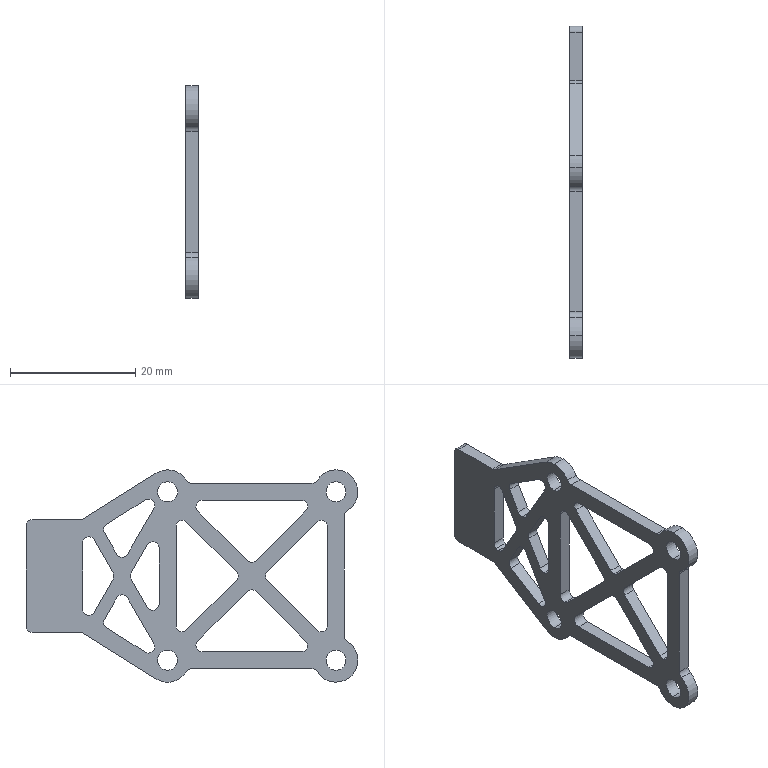Part | SolidWorks | features Extrusion 1, Fillet 1 | 1 solid | 91 faces | box 2 x 52.935 x 33.87 mm | volume 1610 mm3 | cylinder 57 | plane 34 | commonest cylinder face diameters 2 x43 3.2 x8 7 x6